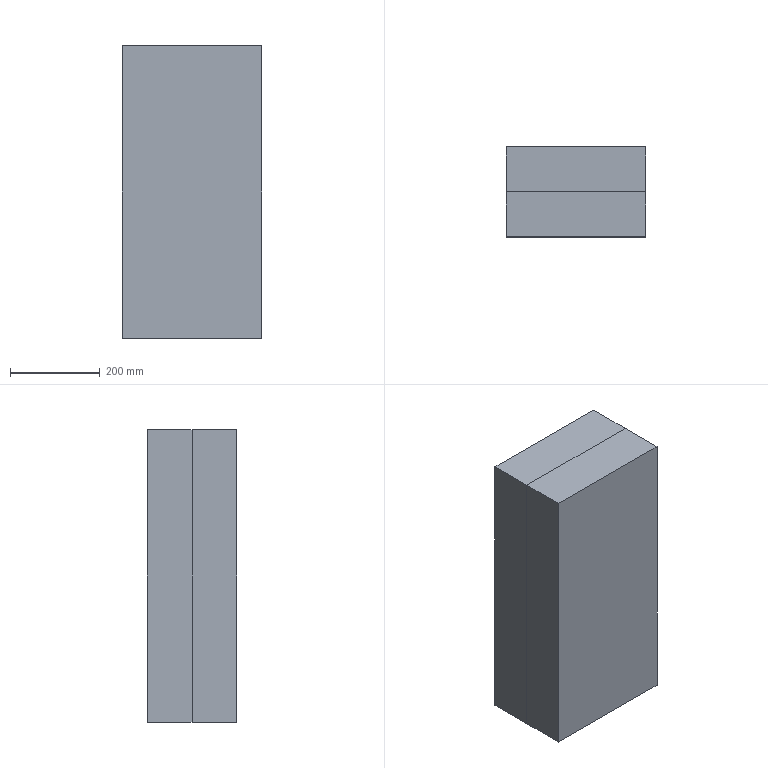Part | 2 solids | 12 faces | box 310 x 200 x 650 mm | volume 40300000 mm3 | plane 12